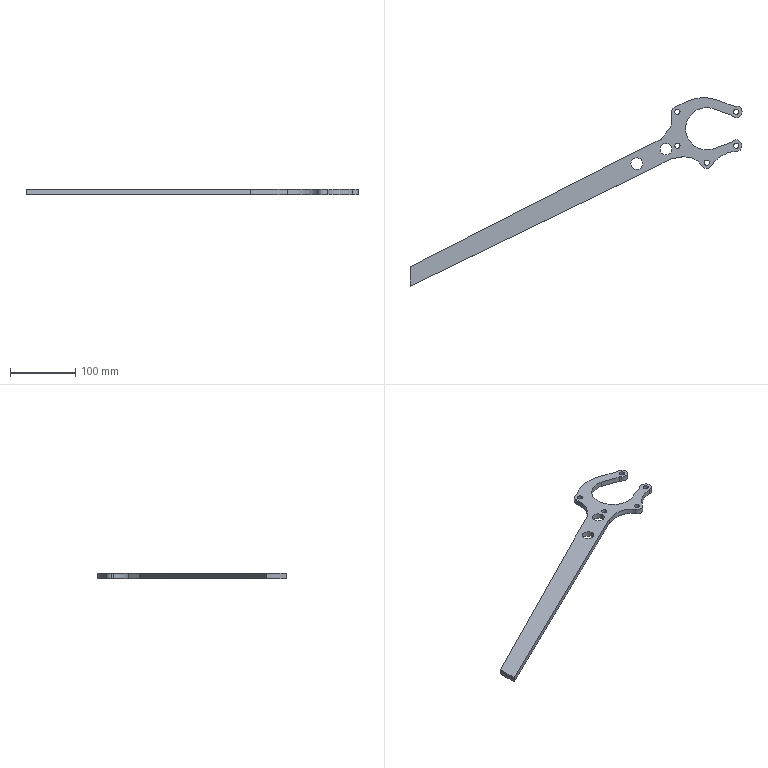Part | SolidWorks | features BaseBody 1 | 1 solid | 39 faces | box 509.458 x 289.148 x 8 mm | volume 145574 mm3 | cylinder 25 | plane 10 | spline 4 | commonest cylinder face diameters 8 x10 18 x9 20 x4 65 x2
STEP:
#1=CARTESIAN_POINT('',(-49.033,-26.,4.));
#2=VERTEX_POINT('',#1);
#3=CARTESIAN_POINT('',(-41.033,-26.,4.));
#4=VERTEX_POINT('',#3);
#5=CARTESIAN_POINT('',(-45.033,-26.,4.));
#6=DIRECTION('',(0.,0.,1.));
#7=DIRECTION('',(-1.,0.,0.));
#8=AXIS2_PLACEMENT_3D('',#5,#6,#7);
#9=CIRCLE('',#8,4.);
#10=EDGE_CURVE('',#2,#4,#9,.T.);
#11=ORIENTED_EDGE('',*,*,#10,.T.);
#12=CARTESIAN_POINT('',(-41.033,-26.,-4.));
#13=VERTEX_POINT('',#12);
#14=CARTESIAN_POINT('',(-41.033,-26.,4.));
#15=DIRECTION('',(0.,0.,-1.));
#16=VECTOR('',#15,1000.);
#17=LINE('',#14,#16);
#18=EDGE_CURVE('',#4,#13,#17,.T.);
#19=ORIENTED_EDGE('',*,*,#18,.T.);
#20=CARTESIAN_POINT('',(-49.033,-26.,-4.));
#21=VERTEX_POINT('',#20);
#22=CARTESIAN_POINT('',(-45.033,-26.,-4.));
#23=DIRECTION('',(0.,0.,-1.));
#24=DIRECTION('',(-1.,0.,0.));
#25=AXIS2_PLACEMENT_3D('',#22,#23,#24);
#26=CIRCLE('',#25,4.);
#27=EDGE_CURVE('',#13,#21,#26,.T.);
#28=ORIENTED_EDGE('',*,*,#27,.T.);
#29=CARTESIAN_POINT('',(-49.033,-26.,4.));
#30=DIRECTION('',(0.,0.,-1.));
#31=VECTOR('',#30,1000.);
#32=LINE('',#29,#31);
#33=EDGE_CURVE('',#2,#21,#32,.T.);
#34=ORIENTED_EDGE('',*,*,#33,.F.);
#35=EDGE_LOOP('',(#11,#19,#28,#34));
#36=FACE_OUTER_BOUND('',#35,.T.);
#37=CARTESIAN_POINT('',(-45.033,-26.,4.));
#38=DIRECTION('',(0.,0.,-1.));
#39=DIRECTION('',(-1.,0.,0.));
#40=AXIS2_PLACEMENT_3D('',#37,#38,#39);
#41=CYLINDRICAL_SURFACE('',#40,4.);
#42=ADVANCED_FACE('',(#36),#41,.F.);
#43=CARTESIAN_POINT('',(49.033,-26.,4.));
#44=VERTEX_POINT('',#43);
#45=CARTESIAN_POINT('',(41.033,-26.,4.));
#46=VERTEX_POINT('',#45);
#47=CARTESIAN_POINT('',(45.033,-26.,4.));
#48=DIRECTION('',(0.,0.,-1.));
#49=DIRECTION('',(-1.,0.,0.));
#50=AXIS2_PLACEMENT_3D('',#47,#48,#49);
#51=CIRCLE('',#50,4.);
#52=EDGE_CURVE('',#44,#46,#51,.T.);
#53=ORIENTED_EDGE('',*,*,#52,.F.);
#54=CARTESIAN_POINT('',(49.033,-26.,-4.));
#55=VERTEX_POINT('',#54);
#56=CARTESIAN_POINT('',(49.033,-26.,4.));
#57=DIRECTION('',(0.,0.,-1.));
#58=VECTOR('',#57,1000.);
#59=LINE('',#56,#58);
#60=EDGE_CURVE('',#44,#55,#59,.T.);
#61=ORIENTED_EDGE('',*,*,#60,.T.);
#62=CARTESIAN_POINT('',(41.033,-26.,-4.));
#63=VERTEX_POINT('',#62);
#64=CARTESIAN_POINT('',(45.033,-26.,-4.));
#65=DIRECTION('',(0.,0.,-1.));
#66=DIRECTION('',(-1.,0.,0.));
#67=AXIS2_PLACEMENT_3D('',#64,#65,#66);
#68=CIRCLE('',#67,4.);
#69=EDGE_CURVE('',#55,#63,#68,.T.);
#70=ORIENTED_EDGE('',*,*,#69,.T.);
#71=CARTESIAN_POINT('',(41.033,-26.,4.));
#72=DIRECTION('',(0.,0.,-1.));
#73=VECTOR('',#72,1000.);
#74=LINE('',#71,#73);
#75=EDGE_CURVE('',#46,#63,#74,.T.);
#76=ORIENTED_EDGE('',*,*,#75,.F.);
#77=EDGE_LOOP('',(#53,#61,#70,#76));
#78=FACE_OUTER_BOUND('',#77,.T.);
#79=CARTESIAN_POINT('',(45.033,-26.,4.));
#80=DIRECTION('',(0.,0.,-1.));
#81=DIRECTION('',(-1.,0.,0.));
#82=AXIS2_PLACEMENT_3D('',#79,#80,#81);
#83=CYLINDRICAL_SURFACE('',#82,4.);
#84=ADVANCED_FACE('',(#78),#83,.F.);
#85=CARTESIAN_POINT('',(4.,-52.,4.));
#86=VERTEX_POINT('',#85);
#87=CARTESIAN_POINT('',(-4.,-52.,4.));
#88=VERTEX_POINT('',#87);
#89=CARTESIAN_POINT('',(0.,-52.,4.));
#90=DIRECTION('',(0.,0.,-1.));
#91=DIRECTION('',(-1.,0.,0.));
#92=AXIS2_PLACEMENT_3D('',#89,#90,#91);
#93=CIRCLE('',#92,4.);
#94=EDGE_CURVE('',#86,#88,#93,.T.);
#95=ORIENTED_EDGE('',*,*,#94,.F.);
#96=CARTESIAN_POINT('',(4.,-52.,-4.));
#97=VERTEX_POINT('',#96);
#98=CARTESIAN_POINT('',(4.,-52.,4.));
#99=DIRECTION('',(0.,0.,-1.));
#100=VECTOR('',#99,1000.);
#101=LINE('',#98,#100);
#102=EDGE_CURVE('',#86,#97,#101,.T.);
#103=ORIENTED_EDGE('',*,*,#102,.T.);
#104=CARTESIAN_POINT('',(-4.,-52.,-4.));
#105=VERTEX_POINT('',#104);
#106=CARTESIAN_POINT('',(0.,-52.,-4.));
#107=DIRECTION('',(0.,0.,-1.));
#108=DIRECTION('',(-1.,0.,0.));
#109=AXIS2_PLACEMENT_3D('',#106,#107,#108);
#110=CIRCLE('',#109,4.);
#111=EDGE_CURVE('',#97,#105,#110,.T.);
#112=ORIENTED_EDGE('',*,*,#111,.T.);
#113=CARTESIAN_POINT('',(-4.,-52.,4.));
#114=DIRECTION('',(0.,0.,-1.));
#115=VECTOR('',#114,1000.);
#116=LINE('',#113,#115);
#117=EDGE_CURVE('',#88,#105,#116,.T.);
#118=ORIENTED_EDGE('',*,*,#117,.F.);
#119=EDGE_LOOP('',(#95,#103,#112,#118));
#120=FACE_OUTER_BOUND('',#119,.T.);
#121=CARTESIAN_POINT('',(0.,-52.,4.));
#122=DIRECTION('',(0.,0.,-1.));
#123=DIRECTION('',(-1.,0.,0.));
#124=AXIS2_PLACEMENT_3D('',#121,#122,#123);
#125=CYLINDRICAL_SURFACE('',#124,4.);
#126=ADVANCED_FACE('',(#120),#125,.F.);
#127=CARTESIAN_POINT('',(49.033,26.,4.));
#128=VERTEX_POINT('',#127);
#129=CARTESIAN_POINT('',(41.033,26.,4.));
#130=VERTEX_POINT('',#129);
#131=CARTESIAN_POINT('',(45.033,26.,4.));
#132=DIRECTION('',(0.,0.,-1.));
#133=DIRECTION('',(-1.,0.,0.));
#134=AXIS2_PLACEMENT_3D('',#131,#132,#133);
#135=CIRCLE('',#134,4.);
#136=EDGE_CURVE('',#128,#130,#135,.T.);
#137=ORIENTED_EDGE('',*,*,#136,.F.);
#138=CARTESIAN_POINT('',(49.033,26.,-4.));
#139=VERTEX_POINT('',#138);
#140=CARTESIAN_POINT('',(49.033,26.,4.));
#141=DIRECTION('',(0.,0.,-1.));
#142=VECTOR('',#141,1000.);
#143=LINE('',#140,#142);
#144=EDGE_CURVE('',#128,#139,#143,.T.);
#145=ORIENTED_EDGE('',*,*,#144,.T.);
#146=CARTESIAN_POINT('',(41.033,26.,-4.));
#147=VERTEX_POINT('',#146);
#148=CARTESIAN_POINT('',(45.033,26.,-4.));
#149=DIRECTION('',(0.,0.,-1.));
#150=DIRECTION('',(-1.,0.,0.));
#151=AXIS2_PLACEMENT_3D('',#148,#149,#150);
#152=CIRCLE('',#151,4.);
#153=EDGE_CURVE('',#139,#147,#152,.T.);
#154=ORIENTED_EDGE('',*,*,#153,.T.);
#155=CARTESIAN_POINT('',(41.033,26.,4.));
#156=DIRECTION('',(0.,0.,-1.));
#157=VECTOR('',#156,1000.);
#158=LINE('',#155,#157);
#159=EDGE_CURVE('',#130,#147,#158,.T.);
#160=ORIENTED_EDGE('',*,*,#159,.F.);
#161=EDGE_LOOP('',(#137,#145,#154,#160));
#162=FACE_OUTER_BOUND('',#161,.T.);
#163=CARTESIAN_POINT('',(45.033,26.,4.));
#164=DIRECTION('',(0.,0.,-1.));
#165=DIRECTION('',(-1.,0.,0.));
#166=AXIS2_PLACEMENT_3D('',#163,#164,#165);
#167=CYLINDRICAL_SURFACE('',#166,4.);
#168=ADVANCED_FACE('',(#162),#167,.F.);
#169=CARTESIAN_POINT('',(-41.033,26.,4.));
#170=VERTEX_POINT('',#169);
#171=CARTESIAN_POINT('',(-49.033,26.,4.));
#172=VERTEX_POINT('',#171);
#173=CARTESIAN_POINT('',(-45.033,26.,4.));
#174=DIRECTION('',(0.,0.,-1.));
#175=DIRECTION('',(-1.,0.,0.));
#176=AXIS2_PLACEMENT_3D('',#173,#174,#175);
#177=CIRCLE('',#176,4.);
#178=EDGE_CURVE('',#170,#172,#177,.T.);
#179=ORIENTED_EDGE('',*,*,#178,.F.);
#180=CARTESIAN_POINT('',(-41.033,26.,-4.));
#181=VERTEX_POINT('',#180);
#182=CARTESIAN_POINT('',(-41.033,26.,4.));
#183=DIRECTION('',(0.,0.,-1.));
#184=VECTOR('',#183,1000.);
#185=LINE('',#182,#184);
#186=EDGE_CURVE('',#170,#181,#185,.T.);
#187=ORIENTED_EDGE('',*,*,#186,.T.);
#188=CARTESIAN_POINT('',(-49.033,26.,-4.));
#189=VERTEX_POINT('',#188);
#190=CARTESIAN_POINT('',(-45.033,26.,-4.));
#191=DIRECTION('',(0.,0.,-1.));
#192=DIRECTION('',(-1.,0.,0.));
#193=AXIS2_PLACEMENT_3D('',#190,#191,#192);
#194=CIRCLE('',#193,4.);
#195=EDGE_CURVE('',#181,#189,#194,.T.);
#196=ORIENTED_EDGE('',*,*,#195,.T.);
#197=CARTESIAN_POINT('',(-49.033,26.,4.));
#198=DIRECTION('',(0.,0.,-1.));
#199=VECTOR('',#198,1000.);
#200=LINE('',#197,#199);
#201=EDGE_CURVE('',#172,#189,#200,.T.);
#202=ORIENTED_EDGE('',*,*,#201,.F.);
#203=EDGE_LOOP('',(#179,#187,#196,#202));
#204=FACE_OUTER_BOUND('',#203,.T.);
#205=CARTESIAN_POINT('',(-45.033,26.,4.));
#206=DIRECTION('',(0.,0.,-1.));
#207=DIRECTION('',(-1.,0.,0.));
#208=AXIS2_PLACEMENT_3D('',#205,#206,#207);
#209=CYLINDRICAL_SURFACE('',#208,4.);
#210=ADVANCED_FACE('',(#204),#209,.F.);
#211=CARTESIAN_POINT('',(-53.645,-31.234,4.));
#212=VERTEX_POINT('',#211);
#213=CARTESIAN_POINT('',(-71.645,-31.234,4.));
#214=VERTEX_POINT('',#213);
#215=CARTESIAN_POINT('',(-62.645,-31.234,4.));
#216=DIRECTION('',(0.,0.,-1.));
#217=DIRECTION('',(-1.,0.,0.));
#218=AXIS2_PLACEMENT_3D('',#215,#216,#217);
#219=CIRCLE('',#218,9.);
#220=EDGE_CURVE('',#212,#214,#219,.T.);
#221=ORIENTED_EDGE('',*,*,#220,.F.);
#222=CARTESIAN_POINT('',(-53.645,-31.234,-4.));
#223=VERTEX_POINT('',#222);
#224=CARTESIAN_POINT('',(-53.645,-31.234,4.));
#225=DIRECTION('',(0.,0.,-1.));
#226=VECTOR('',#225,1000.);
#227=LINE('',#224,#226);
#228=EDGE_CURVE('',#212,#223,#227,.T.);
#229=ORIENTED_EDGE('',*,*,#228,.T.);
#230=CARTESIAN_POINT('',(-71.645,-31.234,-4.));
#231=VERTEX_POINT('',#230);
#232=CARTESIAN_POINT('',(-62.645,-31.234,-4.));
#233=DIRECTION('',(0.,0.,-1.));
#234=DIRECTION('',(-1.,0.,0.));
#235=AXIS2_PLACEMENT_3D('',#232,#233,#234);
#236=CIRCLE('',#235,9.);
#237=EDGE_CURVE('',#223,#231,#236,.T.);
#238=ORIENTED_EDGE('',*,*,#237,.T.);
#239=CARTESIAN_POINT('',(-71.645,-31.234,4.));
#240=DIRECTION('',(0.,0.,-1.));
#241=VECTOR('',#240,1000.);
#242=LINE('',#239,#241);
#243=EDGE_CURVE('',#214,#231,#242,.T.);
#244=ORIENTED_EDGE('',*,*,#243,.F.);
#245=EDGE_LOOP('',(#221,#229,#238,#244));
#246=FACE_OUTER_BOUND('',#245,.T.);
#247=CARTESIAN_POINT('',(-62.645,-31.234,4.));
#248=DIRECTION('',(0.,0.,-1.));
#249=DIRECTION('',(-1.,0.,0.));
#250=AXIS2_PLACEMENT_3D('',#247,#248,#249);
#251=CYLINDRICAL_SURFACE('',#250,9.);
#252=ADVANCED_FACE('',(#246),#251,.F.);
#253=CARTESIAN_POINT('',(-98.392,-53.544,4.));
#254=VERTEX_POINT('',#253);
#255=CARTESIAN_POINT('',(-116.392,-53.544,4.));
#256=VERTEX_POINT('',#255);
#257=CARTESIAN_POINT('',(-107.392,-53.544,4.));
#258=DIRECTION('',(0.,0.,-1.));
#259=DIRECTION('',(-1.,0.,0.));
#260=AXIS2_PLACEMENT_3D('',#257,#258,#259);
#261=CIRCLE('',#260,9.);
#262=EDGE_CURVE('',#254,#256,#261,.T.);
#263=ORIENTED_EDGE('',*,*,#262,.F.);
#264=CARTESIAN_POINT('',(-98.392,-53.544,-4.));
#265=VERTEX_POINT('',#264);
#266=CARTESIAN_POINT('',(-98.392,-53.544,4.));
#267=DIRECTION('',(0.,0.,-1.));
#268=VECTOR('',#267,1000.);
#269=LINE('',#266,#268);
#270=EDGE_CURVE('',#254,#265,#269,.T.);
#271=ORIENTED_EDGE('',*,*,#270,.T.);
#272=CARTESIAN_POINT('',(-116.392,-53.544,-4.));
#273=VERTEX_POINT('',#272);
#274=CARTESIAN_POINT('',(-107.392,-53.544,-4.));
#275=DIRECTION('',(0.,0.,-1.));
#276=DIRECTION('',(-1.,0.,0.));
#277=AXIS2_PLACEMENT_3D('',#274,#275,#276);
#278=CIRCLE('',#277,9.);
#279=EDGE_CURVE('',#265,#273,#278,.T.);
#280=ORIENTED_EDGE('',*,*,#279,.T.);
#281=CARTESIAN_POINT('',(-116.392,-53.544,4.));
#282=DIRECTION('',(0.,0.,-1.));
#283=VECTOR('',#282,1000.);
#284=LINE('',#281,#283);
#285=EDGE_CURVE('',#256,#273,#284,.T.);
#286=ORIENTED_EDGE('',*,*,#285,.F.);
#287=EDGE_LOOP('',(#263,#271,#280,#286));
#288=FACE_OUTER_BOUND('',#287,.T.);
#289=CARTESIAN_POINT('',(-107.392,-53.544,4.));
#290=DIRECTION('',(0.,0.,-1.));
#291=DIRECTION('',(-1.,0.,0.));
#292=AXIS2_PLACEMENT_3D('',#289,#290,#291);
#293=CYLINDRICAL_SURFACE('',#292,9.);
#294=ADVANCED_FACE('',(#288),#293,.F.);
#295=CARTESIAN_POINT('',(-54.033,26.,4.));
#296=VERTEX_POINT('',#295);
#297=CARTESIAN_POINT('',(-53.834,24.118,4.));
#298=VERTEX_POINT('',#297);
#299=CARTESIAN_POINT('',(-45.033,26.,4.));
#300=DIRECTION('',(0.,0.,1.));
#301=DIRECTION('',(-1.,0.,0.));
#302=AXIS2_PLACEMENT_3D('',#299,#300,#301);
#303=CIRCLE('',#302,9.);
#304=EDGE_CURVE('',#296,#298,#303,.T.);
#305=ORIENTED_EDGE('',*,*,#304,.F.);
#306=CARTESIAN_POINT('',(-54.033,26.,-4.));
#307=VERTEX_POINT('',#306);
#308=CARTESIAN_POINT('',(-54.033,26.,4.));
#309=DIRECTION('',(0.,0.,-1.));
#310=VECTOR('',#309,1000.);
#311=LINE('',#308,#310);
#312=EDGE_CURVE('',#296,#307,#311,.T.);
#313=ORIENTED_EDGE('',*,*,#312,.T.);
#314=CARTESIAN_POINT('',(-53.834,24.118,-4.));
#315=VERTEX_POINT('',#314);
#316=CARTESIAN_POINT('',(-45.033,26.,-4.));
#317=DIRECTION('',(0.,0.,1.));
#318=DIRECTION('',(-1.,0.,0.));
#319=AXIS2_PLACEMENT_3D('',#316,#317,#318);
#320=CIRCLE('',#319,9.);
#321=EDGE_CURVE('',#307,#315,#320,.T.);
#322=ORIENTED_EDGE('',*,*,#321,.T.);
#323=CARTESIAN_POINT('',(-53.834,24.118,0.));
#324=DIRECTION('',(0.,0.,1.));
#325=VECTOR('',#324,1000.);
#326=LINE('',#323,#325);
#327=EDGE_CURVE('',#315,#298,#326,.T.);
#328=ORIENTED_EDGE('',*,*,#327,.T.);
#329=EDGE_LOOP('',(#305,#313,#322,#328));
#330=FACE_OUTER_BOUND('',#329,.T.);
#331=CARTESIAN_POINT('',(-45.033,26.,4.));
#332=DIRECTION('',(0.,0.,-1.));
#333=DIRECTION('',(-1.,0.,0.));
#334=AXIS2_PLACEMENT_3D('',#331,#332,#333);
#335=CYLINDRICAL_SURFACE('',#334,9.);
#336=ADVANCED_FACE('',(#330),#335,.T.);
#337=CARTESIAN_POINT('',(-32.5,0.,4.));
#338=VERTEX_POINT('',#337);
#339=CARTESIAN_POINT('',(6.433,31.857,4.));
#340=VERTEX_POINT('',#339);
#341=CARTESIAN_POINT('',(0.,0.,4.));
#342=DIRECTION('',(0.,0.,-1.));
#343=DIRECTION('',(-1.,0.,0.));
#344=AXIS2_PLACEMENT_3D('',#341,#342,#343);
#345=CIRCLE('',#344,32.5);
#346=EDGE_CURVE('',#338,#340,#345,.T.);
#347=ORIENTED_EDGE('',*,*,#346,.F.);
#348=CARTESIAN_POINT('',(-32.5,0.,-4.));
#349=VERTEX_POINT('',#348);
#350=CARTESIAN_POINT('',(-32.5,0.,4.));
#351=DIRECTION('',(0.,0.,-1.));
#352=VECTOR('',#351,1000.);
#353=LINE('',#350,#352);
#354=EDGE_CURVE('',#338,#349,#353,.T.);
#355=ORIENTED_EDGE('',*,*,#354,.T.);
#356=CARTESIAN_POINT('',(6.433,31.857,-4.));
#357=VERTEX_POINT('',#356);
#358=CARTESIAN_POINT('',(0.,0.,-4.));
#359=DIRECTION('',(0.,0.,-1.));
#360=DIRECTION('',(-1.,0.,0.));
#361=AXIS2_PLACEMENT_3D('',#358,#359,#360);
#362=CIRCLE('',#361,32.5);
#363=EDGE_CURVE('',#349,#357,#362,.T.);
#364=ORIENTED_EDGE('',*,*,#363,.T.);
#365=CARTESIAN_POINT('',(6.433,31.857,0.));
#366=DIRECTION('',(0.,0.,-1.));
#367=VECTOR('',#366,1000.);
#368=LINE('',#365,#367);
#369=EDGE_CURVE('',#340,#357,#368,.T.);
#370=ORIENTED_EDGE('',*,*,#369,.F.);
#371=EDGE_LOOP('',(#347,#355,#364,#370));
#372=FACE_OUTER_BOUND('',#371,.T.);
#373=CARTESIAN_POINT('',(0.,0.,4.));
#374=DIRECTION('',(0.,0.,-1.));
#375=DIRECTION('',(-1.,0.,0.));
#376=AXIS2_PLACEMENT_3D('',#373,#374,#375);
#377=CYLINDRICAL_SURFACE('',#376,32.5);
#378=ADVANCED_FACE('',(#372),#377,.F.);
#379=ORIENTED_EDGE('',*,*,#18,.F.);
#380=CARTESIAN_POINT('',(-45.033,-26.,4.));
#381=DIRECTION('',(0.,0.,1.));
#382=DIRECTION('',(-1.,0.,0.));
#383=AXIS2_PLACEMENT_3D('',#380,#381,#382);
#384=CIRCLE('',#383,4.);
#385=EDGE_CURVE('',#4,#2,#384,.T.);
#386=ORIENTED_EDGE('',*,*,#385,.T.);
#387=ORIENTED_EDGE('',*,*,#33,.T.);
#388=CARTESIAN_POINT('',(-45.033,-26.,-4.));
#389=DIRECTION('',(0.,0.,-1.));
#390=DIRECTION('',(-1.,0.,0.));
#391=AXIS2_PLACEMENT_3D('',#388,#389,#390);
#392=CIRCLE('',#391,4.);
#393=EDGE_CURVE('',#21,#13,#392,.T.);
#394=ORIENTED_EDGE('',*,*,#393,.T.);
#395=EDGE_LOOP('',(#379,#386,#387,#394));
#396=FACE_OUTER_BOUND('',#395,.T.);
#397=CARTESIAN_POINT('',(-45.033,-26.,4.));
#398=DIRECTION('',(0.,0.,-1.));
#399=DIRECTION('',(-1.,0.,0.));
#400=AXIS2_PLACEMENT_3D('',#397,#398,#399);
#401=CYLINDRICAL_SURFACE('',#400,4.);
#402=ADVANCED_FACE('',(#396),#401,.F.);
#403=ORIENTED_EDGE('',*,*,#393,.F.);
#404=ORIENTED_EDGE('',*,*,#27,.F.);
#405=EDGE_LOOP('',(#403,#404));
#406=FACE_BOUND('',#405,.T.);
#407=CARTESIAN_POINT('',(45.033,-26.,-4.));
#408=DIRECTION('',(0.,0.,-1.));
#409=DIRECTION('',(-1.,0.,0.));
#410=AXIS2_PLACEMENT_3D('',#407,#408,#409);
#411=CIRCLE('',#410,4.);
#412=EDGE_CURVE('',#63,#55,#411,.T.);
#413=ORIENTED_EDGE('',*,*,#412,.F.);
#414=ORIENTED_EDGE('',*,*,#69,.F.);
#415=EDGE_LOOP('',(#413,#414));
#416=FACE_BOUND('',#415,.T.);
#417=CARTESIAN_POINT('',(0.,-52.,-4.));
#418=DIRECTION('',(0.,0.,-1.));
#419=DIRECTION('',(-1.,0.,0.));
#420=AXIS2_PLACEMENT_3D('',#417,#418,#419);
#421=CIRCLE('',#420,4.);
#422=EDGE_CURVE('',#105,#97,#421,.T.);
#423=ORIENTED_EDGE('',*,*,#422,.F.);
#424=ORIENTED_EDGE('',*,*,#111,.F.);
#425=EDGE_LOOP('',(#423,#424));
#426=FACE_BOUND('',#425,.T.);
#427=CARTESIAN_POINT('',(45.033,26.,-4.));
#428=DIRECTION('',(0.,0.,-1.));
#429=DIRECTION('',(-1.,0.,0.));
#430=AXIS2_PLACEMENT_3D('',#427,#428,#429);
#431=CIRCLE('',#430,4.);
#432=EDGE_CURVE('',#147,#139,#431,.T.);
#433=ORIENTED_EDGE('',*,*,#432,.F.);
#434=ORIENTED_EDGE('',*,*,#153,.F.);
#435=EDGE_LOOP('',(#433,#434));
#436=FACE_BOUND('',#435,.T.);
#437=CARTESIAN_POINT('',(-45.033,26.,-4.));
#438=DIRECTION('',(0.,0.,-1.));
#439=DIRECTION('',(-1.,0.,0.));
#440=AXIS2_PLACEMENT_3D('',#437,#438,#439);
#441=CIRCLE('',#440,4.);
#442=EDGE_CURVE('',#189,#181,#441,.T.);
#443=ORIENTED_EDGE('',*,*,#442,.F.);
#444=ORIENTED_EDGE('',*,*,#195,.F.);
#445=EDGE_LOOP('',(#443,#444));
#446=FACE_BOUND('',#445,.T.);
#447=CARTESIAN_POINT('',(-62.645,-31.234,-4.));
#448=DIRECTION('',(0.,0.,-1.));
#449=DIRECTION('',(-1.,0.,0.));
#450=AXIS2_PLACEMENT_3D('',#447,#448,#449);
#451=CIRCLE('',#450,9.);
#452=EDGE_CURVE('',#231,#223,#451,.T.);
#453=ORIENTED_EDGE('',*,*,#452,.F.);
#454=ORIENTED_EDGE('',*,*,#237,.F.);
#455=EDGE_LOOP('',(#453,#454));
#456=FACE_BOUND('',#455,.T.);
#457=CARTESIAN_POINT('',(-107.392,-53.544,-4.));
#458=DIRECTION('',(0.,0.,-1.));
#459=DIRECTION('',(-1.,0.,0.));
#460=AXIS2_PLACEMENT_3D('',#457,#458,#459);
#461=CIRCLE('',#460,9.);
#462=EDGE_CURVE('',#273,#265,#461,.T.);
#463=ORIENTED_EDGE('',*,*,#462,.F.);
#464=ORIENTED_EDGE('',*,*,#279,.F.);
#465=EDGE_LOOP('',(#463,#464));
#466=FACE_BOUND('',#465,.T.);
#467=CARTESIAN_POINT('',(-455.373,-211.538,-4.));
#468=VERTEX_POINT('',#467);
#469=CARTESIAN_POINT('',(-455.425,-241.465,-4.));
#470=VERTEX_POINT('',#469);
#471=CARTESIAN_POINT('',(-455.425,-241.465,-4.));
#472=DIRECTION('',(-0.001745,-1.,0.));
#473=VECTOR('',#472,1000.);
#474=LINE('',#471,#473);
#475=EDGE_CURVE('',#468,#470,#474,.T.);
#476=ORIENTED_EDGE('',*,*,#475,.F.);
#477=CARTESIAN_POINT('',(-127.298,-44.473,-4.));
#478=VERTEX_POINT('',#477);
#479=CARTESIAN_POINT('',(-455.373,-211.538,-4.));
#480=DIRECTION('',(-0.8911,-0.4538,0.));
#481=VECTOR('',#480,1000.);
#482=LINE('',#479,#481);
#483=EDGE_CURVE('',#478,#468,#482,.T.);
#484=ORIENTED_EDGE('',*,*,#483,.F.);
#485=CARTESIAN_POINT('',(-70.231,-16.02,-4.));
#486=VERTEX_POINT('',#485);
#487=CARTESIAN_POINT('',(-127.298,-44.473,-4.));
#488=DIRECTION('',(-0.8949,-0.4462,0.));
#489=VECTOR('',#488,1000.);
#490=LINE('',#487,#489);
#491=EDGE_CURVE('',#486,#478,#490,.T.);
#492=ORIENTED_EDGE('',*,*,#491,.F.);
#493=CARTESIAN_POINT('',(-57.174,-0.000000019,-4.));
#494=VERTEX_POINT('',#493);
#495=CARTESIAN_POINT('',(-57.174,0.,-4.));
#496=DIRECTION('',(-0.6318,-0.7751,0.));
#497=VECTOR('',#496,1000.);
#498=LINE('',#495,#497);
#499=EDGE_CURVE('',#494,#486,#498,.T.);
#500=ORIENTED_EDGE('',*,*,#499,.F.);
#501=CARTESIAN_POINT('',(-53.834,24.118,-4.));
#502=CARTESIAN_POINT('',(-52.682,12.031,-4.));
#503=CARTESIAN_POINT('',(-54.081,5.475,-4.));
#504=CARTESIAN_POINT('',(-57.174,-0.000000019,-4.));
#505=B_SPLINE_CURVE_WITH_KNOTS('',3,(#501,#502,#503,#504),.UNSPECIFIED.,.F.,.F.,(4,4),(0.,0.02481),.UNSPECIFIED.);
#506=EDGE_CURVE('',#315,#494,#505,.T.);
#507=ORIENTED_EDGE('',*,*,#506,.F.);
#508=ORIENTED_EDGE('',*,*,#321,.F.);
#509=CARTESIAN_POINT('',(-46.406,34.895,-4.));
#510=VERTEX_POINT('',#509);
#511=CARTESIAN_POINT('',(-45.033,26.,-4.));
#512=DIRECTION('',(0.,0.,1.));
#513=DIRECTION('',(-1.,0.,0.));
#514=AXIS2_PLACEMENT_3D('',#511,#512,#513);
#515=CIRCLE('',#514,9.);
#516=EDGE_CURVE('',#510,#307,#515,.T.);
#517=ORIENTED_EDGE('',*,*,#516,.F.);
#518=CARTESIAN_POINT('',(-43.301,35.914,-4.));
#519=VERTEX_POINT('',#518);
#520=CARTESIAN_POINT('',(-47.93,44.778,-4.));
#521=DIRECTION('',(0.,0.,-1.));
#522=DIRECTION('',(-1.,0.,0.));
#523=AXIS2_PLACEMENT_3D('',#520,#521,#522);
#524=CIRCLE('',#523,10.);
#525=EDGE_CURVE('',#519,#510,#524,.T.);
#526=ORIENTED_EDGE('',*,*,#525,.F.);
#527=CARTESIAN_POINT('',(38.851,35.688,-4.));
#528=VERTEX_POINT('',#527);
#529=CARTESIAN_POINT('',(38.851,35.688,-4.));
#530=CARTESIAN_POINT('',(20.692,43.525,-4.));
#531=CARTESIAN_POINT('',(-4.612,51.647,-4.));
#532=CARTESIAN_POINT('',(-28.001,43.905,-4.));
#533=CARTESIAN_POINT('',(-43.301,35.914,-4.));
#534=B_SPLINE_CURVE_WITH_KNOTS('',3,(#529,#530,#531,#532,#533),.UNSPECIFIED.,.F.,.F.,(4,1,4),(0.,0.04398,0.08638),.UNSPECIFIED.);
#535=EDGE_CURVE('',#528,#519,#534,.T.);
#536=ORIENTED_EDGE('',*,*,#535,.F.);
#537=CARTESIAN_POINT('',(43.982,34.938,-4.));
#538=VERTEX_POINT('',#537);
#539=CARTESIAN_POINT('',(42.813,44.87,-4.));
#540=DIRECTION('',(0.,0.,-1.));
#541=DIRECTION('',(-1.,0.,0.));
#542=AXIS2_PLACEMENT_3D('',#539,#540,#541);
#543=CIRCLE('',#542,10.);
#544=EDGE_CURVE('',#538,#528,#543,.T.);
#545=ORIENTED_EDGE('',*,*,#544,.F.);
#546=CARTESIAN_POINT('',(38.803,19.506,-4.));
#547=VERTEX_POINT('',#546);
#548=CARTESIAN_POINT('',(45.033,26.,-4.));
#549=DIRECTION('',(0.,0.,1.));
#550=DIRECTION('',(-1.,0.,0.));
#551=AXIS2_PLACEMENT_3D('',#548,#549,#550);
#552=CIRCLE('',#551,9.);
#553=EDGE_CURVE('',#547,#538,#552,.T.);
#554=ORIENTED_EDGE('',*,*,#553,.F.);
#555=CARTESIAN_POINT('',(35.202,21.721,-4.));
#556=VERTEX_POINT('',#555);
#557=CARTESIAN_POINT('',(31.879,12.29,-4.));
#558=DIRECTION('',(0.,0.,-1.));
#559=DIRECTION('',(-1.,0.,0.));
#560=AXIS2_PLACEMENT_3D('',#557,#558,#559);
#561=CIRCLE('',#560,10.);
#562=EDGE_CURVE('',#556,#547,#561,.T.);
#563=ORIENTED_EDGE('',*,*,#562,.F.);
#564=CARTESIAN_POINT('',(6.433,31.857,-4.));
#565=DIRECTION('',(0.9432,-0.3323,0.));
#566=VECTOR('',#565,1000.);
#567=LINE('',#564,#566);
#568=EDGE_CURVE('',#357,#556,#567,.T.);
#569=ORIENTED_EDGE('',*,*,#568,.F.);
#570=ORIENTED_EDGE('',*,*,#363,.F.);
#571=CARTESIAN_POINT('',(6.433,-31.857,-4.));
#572=VERTEX_POINT('',#571);
#573=CARTESIAN_POINT('',(0.,0.,-4.));
#574=DIRECTION('',(0.,0.,-1.));
#575=DIRECTION('',(-1.,0.,0.));
#576=AXIS2_PLACEMENT_3D('',#573,#574,#575);
#577=CIRCLE('',#576,32.5);
#578=EDGE_CURVE('',#572,#349,#577,.T.);
#579=ORIENTED_EDGE('',*,*,#578,.F.);
#580=CARTESIAN_POINT('',(35.202,-21.721,-4.));
#581=VERTEX_POINT('',#580);
#582=CARTESIAN_POINT('',(6.433,-31.857,-4.));
#583=DIRECTION('',(-0.9432,-0.3323,0.));
#584=VECTOR('',#583,1000.);
#585=LINE('',#582,#584);
#586=EDGE_CURVE('',#581,#572,#585,.T.);
#587=ORIENTED_EDGE('',*,*,#586,.F.);
#588=CARTESIAN_POINT('',(38.803,-19.506,-4.));
#589=VERTEX_POINT('',#588);
#590=CARTESIAN_POINT('',(31.879,-12.29,-4.));
#591=DIRECTION('',(0.,0.,-1.));
#592=DIRECTION('',(-1.,0.,0.));
#593=AXIS2_PLACEMENT_3D('',#590,#591,#592);
#594=CIRCLE('',#593,10.);
#595=EDGE_CURVE('',#589,#581,#594,.T.);
#596=ORIENTED_EDGE('',*,*,#595,.F.);
#597=CARTESIAN_POINT('',(45.033,-35.,-4.));
#598=VERTEX_POINT('',#597);
#599=CARTESIAN_POINT('',(45.033,-26.,-4.));
#600=DIRECTION('',(0.,0.,1.));
#601=DIRECTION('',(-1.,0.,0.));
#602=AXIS2_PLACEMENT_3D('',#599,#600,#601);
#603=CIRCLE('',#602,9.);
#604=EDGE_CURVE('',#598,#589,#603,.T.);
#605=ORIENTED_EDGE('',*,*,#604,.F.);
#606=CARTESIAN_POINT('',(7.645,-56.75,-4.));
#607=VERTEX_POINT('',#606);
#608=CARTESIAN_POINT('',(7.645,-56.75,-4.));
#609=CARTESIAN_POINT('',(14.185,-43.649,-4.));
#610=CARTESIAN_POINT('',(30.699,-34.916,-4.));
#611=CARTESIAN_POINT('',(45.033,-35.,-4.));
#612=B_SPLINE_CURVE_WITH_KNOTS('',3,(#608,#609,#610,#611),.UNSPECIFIED.,.F.,.F.,(4,4),(0.,0.04517),.UNSPECIFIED.);
#613=EDGE_CURVE('',#607,#598,#612,.T.);
#614=ORIENTED_EDGE('',*,*,#613,.F.);
#615=CARTESIAN_POINT('',(-7.645,-56.75,-4.));
#616=VERTEX_POINT('',#615);
#617=CARTESIAN_POINT('',(0.,-52.,-4.));
#618=DIRECTION('',(0.,0.,1.));
#619=DIRECTION('',(-1.,0.,0.));
#620=AXIS2_PLACEMENT_3D('',#617,#618,#619);
#621=CIRCLE('',#620,9.);
#622=EDGE_CURVE('',#616,#607,#621,.T.);
#623=ORIENTED_EDGE('',*,*,#622,.F.);
#624=CARTESIAN_POINT('',(-54.648,-46.242,-4.));
#625=VERTEX_POINT('',#624);
#626=CARTESIAN_POINT('',(-54.648,-46.242,-4.));
#627=CARTESIAN_POINT('',(-20.324,-36.229,-4.));
#628=CARTESIAN_POINT('',(-7.645,-56.75,-4.));
#629=B_SPLINE_CURVE_WITH_KNOTS('',2,(#626,#627,#628),.UNSPECIFIED.,.F.,.F.,(3,3),(0.,0.05204),.UNSPECIFIED.);
#630=EDGE_CURVE('',#625,#616,#629,.T.);
#631=ORIENTED_EDGE('',*,*,#630,.F.);
#632=CARTESIAN_POINT('',(-111.085,-74.381,-4.));
#633=VERTEX_POINT('',#632);
#634=CARTESIAN_POINT('',(-111.085,-74.381,-4.));
#635=DIRECTION('',(0.8949,0.4462,0.));
#636=VECTOR('',#635,1000.);
#637=LINE('',#634,#636);
#638=EDGE_CURVE('',#633,#625,#637,.T.);
#639=ORIENTED_EDGE('',*,*,#638,.F.);
#640=CARTESIAN_POINT('',(-455.425,-241.465,-4.));
#641=DIRECTION('',(0.8997,0.4366,0.));
#642=VECTOR('',#641,1000.);
#643=LINE('',#640,#642);
#644=EDGE_CURVE('',#470,#633,#643,.T.);
#645=ORIENTED_EDGE('',*,*,#644,.F.);
#646=EDGE_LOOP('',(#476,#484,#492,#500,#507,#508,#517,#526,#536,#545,#554,#563,#569,#570,#579,#587,#596,#605,#614,#623,#631,#639,#645));
#647=FACE_OUTER_BOUND('',#646,.T.);
#648=CARTESIAN_POINT('',(-458.482,-243.201,-4.));
#649=DIRECTION('',(0.,0.,1.));
#650=DIRECTION('',(1.,0.,0.));
#651=AXIS2_PLACEMENT_3D('',#648,#649,#650);
#652=PLANE('',#651);
#653=ADVANCED_FACE('',(#406,#416,#426,#436,#446,#456,#466,#647),#652,.F.);
#654=ORIENTED_EDGE('',*,*,#10,.F.);
#655=ORIENTED_EDGE('',*,*,#385,.F.);
#656=EDGE_LOOP('',(#654,#655));
#657=FACE_BOUND('',#656,.T.);
#658=CARTESIAN_POINT('',(45.033,-26.,4.));
#659=DIRECTION('',(0.,0.,-1.));
#660=DIRECTION('',(-1.,0.,0.));
#661=AXIS2_PLACEMENT_3D('',#658,#659,#660);
#662=CIRCLE('',#661,4.);
#663=EDGE_CURVE('',#46,#44,#662,.T.);
#664=ORIENTED_EDGE('',*,*,#663,.T.);
#665=ORIENTED_EDGE('',*,*,#52,.T.);
#666=EDGE_LOOP('',(#664,#665));
#667=FACE_BOUND('',#666,.T.);
#668=CARTESIAN_POINT('',(0.,-52.,4.));
#669=DIRECTION('',(0.,0.,-1.));
#670=DIRECTION('',(-1.,0.,0.));
#671=AXIS2_PLACEMENT_3D('',#668,#669,#670);
#672=CIRCLE('',#671,4.);
#673=EDGE_CURVE('',#88,#86,#672,.T.);
#674=ORIENTED_EDGE('',*,*,#673,.T.);
#675=ORIENTED_EDGE('',*,*,#94,.T.);
#676=EDGE_LOOP('',(#674,#675));
#677=FACE_BOUND('',#676,.T.);
#678=CARTESIAN_POINT('',(45.033,26.,4.));
#679=DIRECTION('',(0.,0.,-1.));
#680=DIRECTION('',(-1.,0.,0.));
#681=AXIS2_PLACEMENT_3D('',#678,#679,#680);
#682=CIRCLE('',#681,4.);
#683=EDGE_CURVE('',#130,#128,#682,.T.);
#684=ORIENTED_EDGE('',*,*,#683,.T.);
#685=ORIENTED_EDGE('',*,*,#136,.T.);
#686=EDGE_LOOP('',(#684,#685));
#687=FACE_BOUND('',#686,.T.);
#688=CARTESIAN_POINT('',(-45.033,26.,4.));
#689=DIRECTION('',(0.,0.,-1.));
#690=DIRECTION('',(-1.,0.,0.));
#691=AXIS2_PLACEMENT_3D('',#688,#689,#690);
#692=CIRCLE('',#691,4.);
#693=EDGE_CURVE('',#172,#170,#692,.T.);
#694=ORIENTED_EDGE('',*,*,#693,.T.);
#695=ORIENTED_EDGE('',*,*,#178,.T.);
#696=EDGE_LOOP('',(#694,#695));
#697=FACE_BOUND('',#696,.T.);
#698=CARTESIAN_POINT('',(-62.645,-31.234,4.));
#699=DIRECTION('',(0.,0.,-1.));
#700=DIRECTION('',(-1.,0.,0.));
#701=AXIS2_PLACEMENT_3D('',#698,#699,#700);
#702=CIRCLE('',#701,9.);
#703=EDGE_CURVE('',#214,#212,#702,.T.);
#704=ORIENTED_EDGE('',*,*,#703,.T.);
#705=ORIENTED_EDGE('',*,*,#220,.T.);
#706=EDGE_LOOP('',(#704,#705));
#707=FACE_BOUND('',#706,.T.);
#708=CARTESIAN_POINT('',(-107.392,-53.544,4.));
#709=DIRECTION('',(0.,0.,-1.));
#710=DIRECTION('',(-1.,0.,0.));
#711=AXIS2_PLACEMENT_3D('',#708,#709,#710);
#712=CIRCLE('',#711,9.);
#713=EDGE_CURVE('',#256,#254,#712,.T.);
#714=ORIENTED_EDGE('',*,*,#713,.T.);
#715=ORIENTED_EDGE('',*,*,#262,.T.);
#716=EDGE_LOOP('',(#714,#715));
#717=FACE_BOUND('',#716,.T.);
#718=CARTESIAN_POINT('',(-70.231,-16.02,4.));
#719=VERTEX_POINT('',#718);
#720=CARTESIAN_POINT('',(-127.298,-44.473,4.));
#721=VERTEX_POINT('',#720);
#722=CARTESIAN_POINT('',(-70.231,-16.02,4.));
#723=DIRECTION('',(-0.8949,-0.4462,0.));
#724=VECTOR('',#723,1000.);
#725=LINE('',#722,#724);
#726=EDGE_CURVE('',#719,#721,#725,.T.);
#727=ORIENTED_EDGE('',*,*,#726,.T.);
#728=CARTESIAN_POINT('',(-455.373,-211.538,4.));
#729=VERTEX_POINT('',#728);
#730=CARTESIAN_POINT('',(-127.298,-44.473,4.));
#731=DIRECTION('',(-0.8911,-0.4538,0.));
#732=VECTOR('',#731,1000.);
#733=LINE('',#730,#732);
#734=EDGE_CURVE('',#721,#729,#733,.T.);
#735=ORIENTED_EDGE('',*,*,#734,.T.);
#736=CARTESIAN_POINT('',(-455.425,-241.465,4.));
#737=VERTEX_POINT('',#736);
#738=CARTESIAN_POINT('',(-455.373,-211.538,4.));
#739=DIRECTION('',(-0.001745,-1.,0.));
#740=VECTOR('',#739,1000.);
#741=LINE('',#738,#740);
#742=EDGE_CURVE('',#729,#737,#741,.T.);
#743=ORIENTED_EDGE('',*,*,#742,.T.);
#744=CARTESIAN_POINT('',(-111.085,-74.381,4.));
#745=VERTEX_POINT('',#744);
#746=CARTESIAN_POINT('',(-455.425,-241.465,4.));
#747=DIRECTION('',(0.8997,0.4366,0.));
#748=VECTOR('',#747,1000.);
#749=LINE('',#746,#748);
#750=EDGE_CURVE('',#737,#745,#749,.T.);
#751=ORIENTED_EDGE('',*,*,#750,.T.);
#752=CARTESIAN_POINT('',(-54.648,-46.242,4.));
#753=VERTEX_POINT('',#752);
#754=CARTESIAN_POINT('',(-111.085,-74.381,4.));
#755=DIRECTION('',(0.8949,0.4462,0.));
#756=VECTOR('',#755,1000.);
#757=LINE('',#754,#756);
#758=EDGE_CURVE('',#745,#753,#757,.T.);
#759=ORIENTED_EDGE('',*,*,#758,.T.);
#760=CARTESIAN_POINT('',(-7.645,-56.75,4.));
#761=VERTEX_POINT('',#760);
#762=CARTESIAN_POINT('',(-54.648,-46.242,4.));
#763=CARTESIAN_POINT('',(-20.324,-36.229,4.));
#764=CARTESIAN_POINT('',(-7.645,-56.75,4.));
#765=B_SPLINE_CURVE_WITH_KNOTS('',2,(#762,#763,#764),.UNSPECIFIED.,.F.,.F.,(3,3),(0.,0.05204),.UNSPECIFIED.);
#766=EDGE_CURVE('',#753,#761,#765,.T.);
#767=ORIENTED_EDGE('',*,*,#766,.T.);
#768=CARTESIAN_POINT('',(7.645,-56.75,4.));
#769=VERTEX_POINT('',#768);
#770=CARTESIAN_POINT('',(0.,-52.,4.));
#771=DIRECTION('',(0.,0.,1.));
#772=DIRECTION('',(-1.,0.,0.));
#773=AXIS2_PLACEMENT_3D('',#770,#771,#772);
#774=CIRCLE('',#773,9.);
#775=EDGE_CURVE('',#761,#769,#774,.T.);
#776=ORIENTED_EDGE('',*,*,#775,.T.);
#777=CARTESIAN_POINT('',(45.033,-35.,4.));
#778=VERTEX_POINT('',#777);
#779=CARTESIAN_POINT('',(7.645,-56.75,4.));
#780=CARTESIAN_POINT('',(14.185,-43.649,4.));
#781=CARTESIAN_POINT('',(30.699,-34.916,4.));
#782=CARTESIAN_POINT('',(45.033,-35.,4.));
#783=B_SPLINE_CURVE_WITH_KNOTS('',3,(#779,#780,#781,#782),.UNSPECIFIED.,.F.,.F.,(4,4),(0.,0.04517),.UNSPECIFIED.);
#784=EDGE_CURVE('',#769,#778,#783,.T.);
#785=ORIENTED_EDGE('',*,*,#784,.T.);
#786=CARTESIAN_POINT('',(38.803,-19.506,4.));
#787=VERTEX_POINT('',#786);
#788=CARTESIAN_POINT('',(45.033,-26.,4.));
#789=DIRECTION('',(0.,0.,1.));
#790=DIRECTION('',(-1.,0.,0.));
#791=AXIS2_PLACEMENT_3D('',#788,#789,#790);
#792=CIRCLE('',#791,9.);
#793=EDGE_CURVE('',#778,#787,#792,.T.);
#794=ORIENTED_EDGE('',*,*,#793,.T.);
#795=CARTESIAN_POINT('',(35.202,-21.721,4.));
#796=VERTEX_POINT('',#795);
#797=CARTESIAN_POINT('',(31.879,-12.29,4.));
#798=DIRECTION('',(0.,0.,-1.));
#799=DIRECTION('',(-1.,0.,0.));
#800=AXIS2_PLACEMENT_3D('',#797,#798,#799);
#801=CIRCLE('',#800,10.);
#802=EDGE_CURVE('',#787,#796,#801,.T.);
#803=ORIENTED_EDGE('',*,*,#802,.T.);
#804=CARTESIAN_POINT('',(6.433,-31.857,4.));
#805=VERTEX_POINT('',#804);
#806=CARTESIAN_POINT('',(35.202,-21.721,4.));
#807=DIRECTION('',(-0.9432,-0.3323,0.));
#808=VECTOR('',#807,1000.);
#809=LINE('',#806,#808);
#810=EDGE_CURVE('',#796,#805,#809,.T.);
#811=ORIENTED_EDGE('',*,*,#810,.T.);
#812=CARTESIAN_POINT('',(0.,0.,4.));
#813=DIRECTION('',(0.,0.,-1.));
#814=DIRECTION('',(-1.,0.,0.));
#815=AXIS2_PLACEMENT_3D('',#812,#813,#814);
#816=CIRCLE('',#815,32.5);
#817=EDGE_CURVE('',#805,#338,#816,.T.);
#818=ORIENTED_EDGE('',*,*,#817,.T.);
#819=ORIENTED_EDGE('',*,*,#346,.T.);
#820=CARTESIAN_POINT('',(35.202,21.721,4.));
#821=VERTEX_POINT('',#820);
#822=CARTESIAN_POINT('',(6.433,31.857,4.));
#823=DIRECTION('',(0.9432,-0.3323,0.));
#824=VECTOR('',#823,1000.);
#825=LINE('',#822,#824);
#826=EDGE_CURVE('',#340,#821,#825,.T.);
#827=ORIENTED_EDGE('',*,*,#826,.T.);
#828=CARTESIAN_POINT('',(38.803,19.506,4.));
#829=VERTEX_POINT('',#828);
#830=CARTESIAN_POINT('',(31.879,12.29,4.));
#831=DIRECTION('',(0.,0.,-1.));
#832=DIRECTION('',(-1.,0.,0.));
#833=AXIS2_PLACEMENT_3D('',#830,#831,#832);
#834=CIRCLE('',#833,10.);
#835=EDGE_CURVE('',#821,#829,#834,.T.);
#836=ORIENTED_EDGE('',*,*,#835,.T.);
#837=CARTESIAN_POINT('',(43.982,34.938,4.));
#838=VERTEX_POINT('',#837);
#839=CARTESIAN_POINT('',(45.033,26.,4.));
#840=DIRECTION('',(0.,0.,1.));
#841=DIRECTION('',(-1.,0.,0.));
#842=AXIS2_PLACEMENT_3D('',#839,#840,#841);
#843=CIRCLE('',#842,9.);
#844=EDGE_CURVE('',#829,#838,#843,.T.);
#845=ORIENTED_EDGE('',*,*,#844,.T.);
#846=CARTESIAN_POINT('',(38.851,35.688,4.));
#847=VERTEX_POINT('',#846);
#848=CARTESIAN_POINT('',(42.813,44.87,4.));
#849=DIRECTION('',(0.,0.,-1.));
#850=DIRECTION('',(-1.,0.,0.));
#851=AXIS2_PLACEMENT_3D('',#848,#849,#850);
#852=CIRCLE('',#851,10.);
#853=EDGE_CURVE('',#838,#847,#852,.T.);
#854=ORIENTED_EDGE('',*,*,#853,.T.);
#855=CARTESIAN_POINT('',(-43.301,35.914,4.));
#856=VERTEX_POINT('',#855);
#857=CARTESIAN_POINT('',(38.851,35.688,4.));
#858=CARTESIAN_POINT('',(20.692,43.525,4.));
#859=CARTESIAN_POINT('',(-4.612,51.647,4.));
#860=CARTESIAN_POINT('',(-28.001,43.905,4.));
#861=CARTESIAN_POINT('',(-43.301,35.914,4.));
#862=B_SPLINE_CURVE_WITH_KNOTS('',3,(#857,#858,#859,#860,#861),.UNSPECIFIED.,.F.,.F.,(4,1,4),(0.,0.04398,0.08638),.UNSPECIFIED.);
#863=EDGE_CURVE('',#847,#856,#862,.T.);
#864=ORIENTED_EDGE('',*,*,#863,.T.);
#865=CARTESIAN_POINT('',(-46.406,34.895,4.));
#866=VERTEX_POINT('',#865);
#867=CARTESIAN_POINT('',(-47.93,44.778,4.));
#868=DIRECTION('',(0.,0.,-1.));
#869=DIRECTION('',(-1.,0.,0.));
#870=AXIS2_PLACEMENT_3D('',#867,#868,#869);
#871=CIRCLE('',#870,10.);
#872=EDGE_CURVE('',#856,#866,#871,.T.);
#873=ORIENTED_EDGE('',*,*,#872,.T.);
#874=CARTESIAN_POINT('',(-45.033,26.,4.));
#875=DIRECTION('',(0.,0.,1.));
#876=DIRECTION('',(-1.,0.,0.));
#877=AXIS2_PLACEMENT_3D('',#874,#875,#876);
#878=CIRCLE('',#877,9.);
#879=EDGE_CURVE('',#866,#296,#878,.T.);
#880=ORIENTED_EDGE('',*,*,#879,.T.);
#881=ORIENTED_EDGE('',*,*,#304,.T.);
#882=CARTESIAN_POINT('',(-57.174,-0.000000015,4.));
#883=VERTEX_POINT('',#882);
#884=CARTESIAN_POINT('',(-53.834,24.118,4.));
#885=CARTESIAN_POINT('',(-52.682,12.031,4.));
#886=CARTESIAN_POINT('',(-54.081,5.475,4.));
#887=CARTESIAN_POINT('',(-57.174,-0.000000015,4.));
#888=B_SPLINE_CURVE_WITH_KNOTS('',3,(#884,#885,#886,#887),.UNSPECIFIED.,.F.,.F.,(4,4),(0.,0.02481),.UNSPECIFIED.);
#889=EDGE_CURVE('',#298,#883,#888,.T.);
#890=ORIENTED_EDGE('',*,*,#889,.T.);
#891=CARTESIAN_POINT('',(-57.174,-0.000000053,4.));
#892=DIRECTION('',(-0.6318,-0.7751,0.));
#893=VECTOR('',#892,1000.);
#894=LINE('',#891,#893);
#895=EDGE_CURVE('',#883,#719,#894,.T.);
#896=ORIENTED_EDGE('',*,*,#895,.T.);
#897=EDGE_LOOP('',(#727,#735,#743,#751,#759,#767,#776,#785,#794,#803,#811,#818,#819,#827,#836,#845,#854,#864,#873,#880,#881,#890,#896));
#898=FACE_OUTER_BOUND('',#897,.T.);
#899=CARTESIAN_POINT('',(-458.482,-243.201,4.));
#900=DIRECTION('',(0.,0.,1.));
#901=DIRECTION('',(1.,0.,0.));
#902=AXIS2_PLACEMENT_3D('',#899,#900,#901);
#903=PLANE('',#902);
#904=ADVANCED_FACE('',(#657,#667,#677,#687,#697,#707,#717,#898),#903,.T.);
#905=ORIENTED_EDGE('',*,*,#60,.F.);
#906=ORIENTED_EDGE('',*,*,#663,.F.);
#907=ORIENTED_EDGE('',*,*,#75,.T.);
#908=ORIENTED_EDGE('',*,*,#412,.T.);
#909=EDGE_LOOP('',(#905,#906,#907,#908));
#910=FACE_OUTER_BOUND('',#909,.T.);
#911=CARTESIAN_POINT('',(45.033,-26.,4.));
#912=DIRECTION('',(0.,0.,-1.));
#913=DIRECTION('',(-1.,0.,0.));
#914=AXIS2_PLACEMENT_3D('',#911,#912,#913);
#915=CYLINDRICAL_SURFACE('',#914,4.);
#916=ADVANCED_FACE('',(#910),#915,.F.);
#917=ORIENTED_EDGE('',*,*,#102,.F.);
#918=ORIENTED_EDGE('',*,*,#673,.F.);
#919=ORIENTED_EDGE('',*,*,#117,.T.);
#920=ORIENTED_EDGE('',*,*,#422,.T.);
#921=EDGE_LOOP('',(#917,#918,#919,#920));
#922=FACE_OUTER_BOUND('',#921,.T.);
#923=CARTESIAN_POINT('',(0.,-52.,4.));
#924=DIRECTION('',(0.,0.,-1.));
#925=DIRECTION('',(-1.,0.,0.));
#926=AXIS2_PLACEMENT_3D('',#923,#924,#925);
#927=CYLINDRICAL_SURFACE('',#926,4.);
#928=ADVANCED_FACE('',(#922),#927,.F.);
#929=ORIENTED_EDGE('',*,*,#144,.F.);
#930=ORIENTED_EDGE('',*,*,#683,.F.);
#931=ORIENTED_EDGE('',*,*,#159,.T.);
#932=ORIENTED_EDGE('',*,*,#432,.T.);
#933=EDGE_LOOP('',(#929,#930,#931,#932));
#934=FACE_OUTER_BOUND('',#933,.T.);
#935=CARTESIAN_POINT('',(45.033,26.,4.));
#936=DIRECTION('',(0.,0.,-1.));
#937=DIRECTION('',(-1.,0.,0.));
#938=AXIS2_PLACEMENT_3D('',#935,#936,#937);
#939=CYLINDRICAL_SURFACE('',#938,4.);
#940=ADVANCED_FACE('',(#934),#939,.F.);
#941=ORIENTED_EDGE('',*,*,#186,.F.);
#942=ORIENTED_EDGE('',*,*,#693,.F.);
#943=ORIENTED_EDGE('',*,*,#201,.T.);
#944=ORIENTED_EDGE('',*,*,#442,.T.);
#945=EDGE_LOOP('',(#941,#942,#943,#944));
#946=FACE_OUTER_BOUND('',#945,.T.);
#947=CARTESIAN_POINT('',(-45.033,26.,4.));
#948=DIRECTION('',(0.,0.,-1.));
#949=DIRECTION('',(-1.,0.,0.));
#950=AXIS2_PLACEMENT_3D('',#947,#948,#949);
#951=CYLINDRICAL_SURFACE('',#950,4.);
#952=ADVANCED_FACE('',(#946),#951,.F.);
#953=ORIENTED_EDGE('',*,*,#228,.F.);
#954=ORIENTED_EDGE('',*,*,#703,.F.);
#955=ORIENTED_EDGE('',*,*,#243,.T.);
#956=ORIENTED_EDGE('',*,*,#452,.T.);
#957=EDGE_LOOP('',(#953,#954,#955,#956));
#958=FACE_OUTER_BOUND('',#957,.T.);
#959=CARTESIAN_POINT('',(-62.645,-31.234,4.));
#960=DIRECTION('',(0.,0.,-1.));
#961=DIRECTION('',(-1.,0.,0.));
#962=AXIS2_PLACEMENT_3D('',#959,#960,#961);
#963=CYLINDRICAL_SURFACE('',#962,9.);
#964=ADVANCED_FACE('',(#958),#963,.F.);
#965=ORIENTED_EDGE('',*,*,#270,.F.);
#966=ORIENTED_EDGE('',*,*,#713,.F.);
#967=ORIENTED_EDGE('',*,*,#285,.T.);
#968=ORIENTED_EDGE('',*,*,#462,.T.);
#969=EDGE_LOOP('',(#965,#966,#967,#968));
#970=FACE_OUTER_BOUND('',#969,.T.);
#971=CARTESIAN_POINT('',(-107.392,-53.544,4.));
#972=DIRECTION('',(0.,0.,-1.));
#973=DIRECTION('',(-1.,0.,0.));
#974=AXIS2_PLACEMENT_3D('',#971,#972,#973);
#975=CYLINDRICAL_SURFACE('',#974,9.);
#976=ADVANCED_FACE('',(#970),#975,.F.);
#977=CARTESIAN_POINT('',(-111.085,-74.381,0.));
#978=DIRECTION('',(0.,0.,1.));
#979=VECTOR('',#978,1000.);
#980=LINE('',#977,#979);
#981=EDGE_CURVE('',#633,#745,#980,.T.);
#982=ORIENTED_EDGE('',*,*,#981,.T.);
#983=ORIENTED_EDGE('',*,*,#750,.F.);
#984=CARTESIAN_POINT('',(-455.425,-241.465,0.));
#985=DIRECTION('',(0.,0.,-1.));
#986=VECTOR('',#985,1000.);
#987=LINE('',#984,#986);
#988=EDGE_CURVE('',#737,#470,#987,.T.);
#989=ORIENTED_EDGE('',*,*,#988,.T.);
#990=ORIENTED_EDGE('',*,*,#644,.T.);
#991=EDGE_LOOP('',(#982,#983,#989,#990));
#992=FACE_OUTER_BOUND('',#991,.T.);
#993=CARTESIAN_POINT('',(-455.425,-241.465,-4.));
#994=DIRECTION('',(0.4366,-0.8997,0.));
#995=DIRECTION('',(0.8997,0.4366,0.));
#996=AXIS2_PLACEMENT_3D('',#993,#994,#995);
#997=PLANE('',#996);
#998=ADVANCED_FACE('',(#992),#997,.T.);
#999=ORIENTED_EDGE('',*,*,#988,.F.);
#1000=ORIENTED_EDGE('',*,*,#742,.F.);
#1001=CARTESIAN_POINT('',(-455.373,-211.538,0.));
#1002=DIRECTION('',(0.,0.,1.));
#1003=VECTOR('',#1002,1000.);
#1004=LINE('',#1001,#1003);
#1005=EDGE_CURVE('',#468,#729,#1004,.T.);
#1006=ORIENTED_EDGE('',*,*,#1005,.F.);
#1007=ORIENTED_EDGE('',*,*,#475,.T.);
#1008=EDGE_LOOP('',(#999,#1000,#1006,#1007));
#1009=FACE_OUTER_BOUND('',#1008,.T.);
#1010=CARTESIAN_POINT('',(-455.425,-241.465,-4.));
#1011=DIRECTION('',(1.,-0.001745,0.));
#1012=DIRECTION('',(0.001745,1.,0.));
#1013=AXIS2_PLACEMENT_3D('',#1010,#1011,#1012);
#1014=PLANE('',#1013);
#1015=ADVANCED_FACE('',(#1009),#1014,.F.);
#1016=ORIENTED_EDGE('',*,*,#1005,.T.);
#1017=ORIENTED_EDGE('',*,*,#734,.F.);
#1018=CARTESIAN_POINT('',(-127.298,-44.473,0.));
#1019=DIRECTION('',(0.,0.,1.));
#1020=VECTOR('',#1019,1000.);
#1021=LINE('',#1018,#1020);
#1022=EDGE_CURVE('',#478,#721,#1021,.T.);
#1023=ORIENTED_EDGE('',*,*,#1022,.F.);
#1024=ORIENTED_EDGE('',*,*,#483,.T.);
#1025=EDGE_LOOP('',(#1016,#1017,#1023,#1024));
#1026=FACE_OUTER_BOUND('',#1025,.T.);
#1027=CARTESIAN_POINT('',(-455.373,-211.538,-4.));
#1028=DIRECTION('',(0.4538,-0.8911,0.));
#1029=DIRECTION('',(0.8911,0.4538,0.));
#1030=AXIS2_PLACEMENT_3D('',#1027,#1028,#1029);
#1031=PLANE('',#1030);
#1032=ADVANCED_FACE('',(#1026),#1031,.F.);
#1033=ORIENTED_EDGE('',*,*,#1022,.T.);
#1034=ORIENTED_EDGE('',*,*,#726,.F.);
#1035=CARTESIAN_POINT('',(-70.231,-16.02,0.));
#1036=DIRECTION('',(0.,0.,1.));
#1037=VECTOR('',#1036,1000.);
#1038=LINE('',#1035,#1037);
#1039=EDGE_CURVE('',#486,#719,#1038,.T.);
#1040=ORIENTED_EDGE('',*,*,#1039,.F.);
#1041=ORIENTED_EDGE('',*,*,#491,.T.);
#1042=EDGE_LOOP('',(#1033,#1034,#1040,#1041));
#1043=FACE_OUTER_BOUND('',#1042,.T.);
#1044=CARTESIAN_POINT('',(-127.298,-44.473,-4.));
#1045=DIRECTION('',(0.4462,-0.8949,0.));
#1046=DIRECTION('',(0.8949,0.4462,0.));
#1047=AXIS2_PLACEMENT_3D('',#1044,#1045,#1046);
#1048=PLANE('',#1047);
#1049=ADVANCED_FACE('',(#1043),#1048,.F.);
#1050=ORIENTED_EDGE('',*,*,#895,.F.);
#1051=CARTESIAN_POINT('',(-57.174,0.,0.));
#1052=DIRECTION('',(0.,0.,-1.));
#1053=VECTOR('',#1052,1000.);
#1054=LINE('',#1051,#1053);
#1055=EDGE_CURVE('',#883,#494,#1054,.T.);
#1056=ORIENTED_EDGE('',*,*,#1055,.T.);
#1057=ORIENTED_EDGE('',*,*,#499,.T.);
#1058=ORIENTED_EDGE('',*,*,#1039,.T.);
#1059=EDGE_LOOP('',(#1050,#1056,#1057,#1058));
#1060=FACE_OUTER_BOUND('',#1059,.T.);
#1061=CARTESIAN_POINT('',(-57.174,0.,-4.));
#1062=DIRECTION('',(-0.7751,0.6318,0.));
#1063=DIRECTION('',(-0.6318,-0.7751,0.));
#1064=AXIS2_PLACEMENT_3D('',#1061,#1062,#1063);
#1065=PLANE('',#1064);
#1066=ADVANCED_FACE('',(#1060),#1065,.T.);
#1067=ORIENTED_EDGE('',*,*,#1055,.F.);
#1068=ORIENTED_EDGE('',*,*,#889,.F.);
#1069=ORIENTED_EDGE('',*,*,#327,.F.);
#1070=ORIENTED_EDGE('',*,*,#506,.T.);
#1071=EDGE_LOOP('',(#1067,#1068,#1069,#1070));
#1072=FACE_OUTER_BOUND('',#1071,.T.);
#1073=CARTESIAN_POINT('',(-53.834,24.118,4.));
#1074=CARTESIAN_POINT('',(-53.834,24.118,-4.));
#1075=CARTESIAN_POINT('',(-52.682,12.031,4.));
#1076=CARTESIAN_POINT('',(-52.682,12.031,-4.));
#1077=CARTESIAN_POINT('',(-54.081,5.475,4.));
#1078=CARTESIAN_POINT('',(-54.081,5.475,-4.));
#1079=CARTESIAN_POINT('',(-57.174,0.,4.));
#1080=CARTESIAN_POINT('',(-57.174,0.,-4.));
#1081=B_SPLINE_SURFACE_WITH_KNOTS('',3,1,((#1073,#1074),(#1075,#1076),(#1077,#1078),(#1079,#1080)),.UNSPECIFIED.,.F.,.F.,.F.,(4,4),(2,2),(0.,1.),(0.,1.),.UNSPECIFIED.);
#1082=ADVANCED_FACE('',(#1072),#1081,.F.);
#1083=ORIENTED_EDGE('',*,*,#312,.F.);
#1084=ORIENTED_EDGE('',*,*,#879,.F.);
#1085=CARTESIAN_POINT('',(-46.406,34.895,0.));
#1086=DIRECTION('',(0.,0.,1.));
#1087=VECTOR('',#1086,1000.);
#1088=LINE('',#1085,#1087);
#1089=EDGE_CURVE('',#510,#866,#1088,.T.);
#1090=ORIENTED_EDGE('',*,*,#1089,.F.);
#1091=ORIENTED_EDGE('',*,*,#516,.T.);
#1092=EDGE_LOOP('',(#1083,#1084,#1090,#1091));
#1093=FACE_OUTER_BOUND('',#1092,.T.);
#1094=CARTESIAN_POINT('',(-45.033,26.,4.));
#1095=DIRECTION('',(0.,0.,-1.));
#1096=DIRECTION('',(-1.,0.,0.));
#1097=AXIS2_PLACEMENT_3D('',#1094,#1095,#1096);
#1098=CYLINDRICAL_SURFACE('',#1097,9.);
#1099=ADVANCED_FACE('',(#1093),#1098,.T.);
#1100=ORIENTED_EDGE('',*,*,#872,.F.);
#1101=CARTESIAN_POINT('',(-43.301,35.914,0.));
#1102=DIRECTION('',(0.,0.,-1.));
#1103=VECTOR('',#1102,1000.);
#1104=LINE('',#1101,#1103);
#1105=EDGE_CURVE('',#856,#519,#1104,.T.);
#1106=ORIENTED_EDGE('',*,*,#1105,.T.);
#1107=ORIENTED_EDGE('',*,*,#525,.T.);
#1108=ORIENTED_EDGE('',*,*,#1089,.T.);
#1109=EDGE_LOOP('',(#1100,#1106,#1107,#1108));
#1110=FACE_OUTER_BOUND('',#1109,.T.);
#1111=CARTESIAN_POINT('',(-47.93,44.778,4.));
#1112=DIRECTION('',(0.,0.,-1.));
#1113=DIRECTION('',(-1.,0.,0.));
#1114=AXIS2_PLACEMENT_3D('',#1111,#1112,#1113);
#1115=CYLINDRICAL_SURFACE('',#1114,10.);
#1116=ADVANCED_FACE('',(#1110),#1115,.F.);
#1117=ORIENTED_EDGE('',*,*,#1105,.F.);
#1118=ORIENTED_EDGE('',*,*,#863,.F.);
#1119=CARTESIAN_POINT('',(38.851,35.688,0.));
#1120=DIRECTION('',(0.,0.,1.));
#1121=VECTOR('',#1120,1000.);
#1122=LINE('',#1119,#1121);
#1123=EDGE_CURVE('',#528,#847,#1122,.T.);
#1124=ORIENTED_EDGE('',*,*,#1123,.F.);
#1125=ORIENTED_EDGE('',*,*,#535,.T.);
#1126=EDGE_LOOP('',(#1117,#1118,#1124,#1125));
#1127=FACE_OUTER_BOUND('',#1126,.T.);
#1128=CARTESIAN_POINT('',(38.851,35.688,4.));
#1129=CARTESIAN_POINT('',(38.851,35.688,-4.));
#1130=CARTESIAN_POINT('',(38.851,35.688,4.));
#1131=CARTESIAN_POINT('',(38.851,35.688,-4.));
#1132=CARTESIAN_POINT('',(38.851,35.688,4.));
#1133=CARTESIAN_POINT('',(38.851,35.688,-4.));
#1134=CARTESIAN_POINT('',(38.851,35.688,4.));
#1135=CARTESIAN_POINT('',(38.851,35.688,-4.));
#1136=CARTESIAN_POINT('',(20.692,43.525,4.));
#1137=CARTESIAN_POINT('',(20.692,43.525,-4.));
#1138=CARTESIAN_POINT('',(-4.612,51.647,4.));
#1139=CARTESIAN_POINT('',(-4.612,51.647,-4.));
#1140=CARTESIAN_POINT('',(-28.001,43.905,4.));
#1141=CARTESIAN_POINT('',(-28.001,43.905,-4.));
#1142=CARTESIAN_POINT('',(-43.301,35.914,4.));
#1143=CARTESIAN_POINT('',(-43.301,35.914,-4.));
#1144=B_SPLINE_SURFACE_WITH_KNOTS('',3,1,((#1128,#1129),(#1130,#1131),(#1132,#1133),(#1134,#1135),(#1136,#1137),(#1138,#1139),(#1140,#1141),(#1142,#1143)),.UNSPECIFIED.,.F.,.F.,.F.,(4,3,1,4),(2,2),(0.026,0.02601,0.513,0.9824),(0.,1.),.UNSPECIFIED.);
#1145=ADVANCED_FACE('',(#1127),#1144,.F.);
#1146=ORIENTED_EDGE('',*,*,#853,.F.);
#1147=CARTESIAN_POINT('',(43.982,34.938,0.));
#1148=DIRECTION('',(0.,0.,-1.));
#1149=VECTOR('',#1148,1000.);
#1150=LINE('',#1147,#1149);
#1151=EDGE_CURVE('',#838,#538,#1150,.T.);
#1152=ORIENTED_EDGE('',*,*,#1151,.T.);
#1153=ORIENTED_EDGE('',*,*,#544,.T.);
#1154=ORIENTED_EDGE('',*,*,#1123,.T.);
#1155=EDGE_LOOP('',(#1146,#1152,#1153,#1154));
#1156=FACE_OUTER_BOUND('',#1155,.T.);
#1157=CARTESIAN_POINT('',(42.813,44.87,4.));
#1158=DIRECTION('',(0.,0.,-1.));
#1159=DIRECTION('',(-1.,0.,0.));
#1160=AXIS2_PLACEMENT_3D('',#1157,#1158,#1159);
#1161=CYLINDRICAL_SURFACE('',#1160,10.);
#1162=ADVANCED_FACE('',(#1156),#1161,.F.);
#1163=ORIENTED_EDGE('',*,*,#1151,.F.);
#1164=ORIENTED_EDGE('',*,*,#844,.F.);
#1165=CARTESIAN_POINT('',(38.803,19.506,0.));
#1166=DIRECTION('',(0.,0.,1.));
#1167=VECTOR('',#1166,1000.);
#1168=LINE('',#1165,#1167);
#1169=EDGE_CURVE('',#547,#829,#1168,.T.);
#1170=ORIENTED_EDGE('',*,*,#1169,.F.);
#1171=ORIENTED_EDGE('',*,*,#553,.T.);
#1172=EDGE_LOOP('',(#1163,#1164,#1170,#1171));
#1173=FACE_OUTER_BOUND('',#1172,.T.);
#1174=CARTESIAN_POINT('',(45.033,26.,4.));
#1175=DIRECTION('',(0.,0.,-1.));
#1176=DIRECTION('',(-1.,0.,0.));
#1177=AXIS2_PLACEMENT_3D('',#1174,#1175,#1176);
#1178=CYLINDRICAL_SURFACE('',#1177,9.);
#1179=ADVANCED_FACE('',(#1173),#1178,.T.);
#1180=ORIENTED_EDGE('',*,*,#835,.F.);
#1181=CARTESIAN_POINT('',(35.202,21.721,0.));
#1182=DIRECTION('',(0.,0.,-1.));
#1183=VECTOR('',#1182,1000.);
#1184=LINE('',#1181,#1183);
#1185=EDGE_CURVE('',#821,#556,#1184,.T.);
#1186=ORIENTED_EDGE('',*,*,#1185,.T.);
#1187=ORIENTED_EDGE('',*,*,#562,.T.);
#1188=ORIENTED_EDGE('',*,*,#1169,.T.);
#1189=EDGE_LOOP('',(#1180,#1186,#1187,#1188));
#1190=FACE_OUTER_BOUND('',#1189,.T.);
#1191=CARTESIAN_POINT('',(31.879,12.29,4.));
#1192=DIRECTION('',(0.,0.,-1.));
#1193=DIRECTION('',(-1.,0.,0.));
#1194=AXIS2_PLACEMENT_3D('',#1191,#1192,#1193);
#1195=CYLINDRICAL_SURFACE('',#1194,10.);
#1196=ADVANCED_FACE('',(#1190),#1195,.F.);
#1197=ORIENTED_EDGE('',*,*,#826,.F.);
#1198=ORIENTED_EDGE('',*,*,#369,.T.);
#1199=ORIENTED_EDGE('',*,*,#568,.T.);
#1200=ORIENTED_EDGE('',*,*,#1185,.F.);
#1201=EDGE_LOOP('',(#1197,#1198,#1199,#1200));
#1202=FACE_OUTER_BOUND('',#1201,.T.);
#1203=CARTESIAN_POINT('',(6.433,31.857,-4.));
#1204=DIRECTION('',(-0.3323,-0.9432,0.));
#1205=DIRECTION('',(0.9432,-0.3323,0.));
#1206=AXIS2_PLACEMENT_3D('',#1203,#1204,#1205);
#1207=PLANE('',#1206);
#1208=ADVANCED_FACE('',(#1202),#1207,.T.);
#1209=ORIENTED_EDGE('',*,*,#354,.F.);
#1210=ORIENTED_EDGE('',*,*,#817,.F.);
#1211=CARTESIAN_POINT('',(6.433,-31.857,0.));
#1212=DIRECTION('',(0.,0.,-1.));
#1213=VECTOR('',#1212,1000.);
#1214=LINE('',#1211,#1213);
#1215=EDGE_CURVE('',#805,#572,#1214,.T.);
#1216=ORIENTED_EDGE('',*,*,#1215,.T.);
#1217=ORIENTED_EDGE('',*,*,#578,.T.);
#1218=EDGE_LOOP('',(#1209,#1210,#1216,#1217));
#1219=FACE_OUTER_BOUND('',#1218,.T.);
#1220=CARTESIAN_POINT('',(0.,0.,4.));
#1221=DIRECTION('',(0.,0.,-1.));
#1222=DIRECTION('',(-1.,0.,0.));
#1223=AXIS2_PLACEMENT_3D('',#1220,#1221,#1222);
#1224=CYLINDRICAL_SURFACE('',#1223,32.5);
#1225=ADVANCED_FACE('',(#1219),#1224,.F.);
#1226=ORIENTED_EDGE('',*,*,#1215,.F.);
#1227=ORIENTED_EDGE('',*,*,#810,.F.);
#1228=CARTESIAN_POINT('',(35.202,-21.721,0.));
#1229=DIRECTION('',(0.,0.,1.));
#1230=VECTOR('',#1229,1000.);
#1231=LINE('',#1228,#1230);
#1232=EDGE_CURVE('',#581,#796,#1231,.T.);
#1233=ORIENTED_EDGE('',*,*,#1232,.F.);
#1234=ORIENTED_EDGE('',*,*,#586,.T.);
#1235=EDGE_LOOP('',(#1226,#1227,#1233,#1234));
#1236=FACE_OUTER_BOUND('',#1235,.T.);
#1237=CARTESIAN_POINT('',(6.433,-31.857,-4.));
#1238=DIRECTION('',(0.3323,-0.9432,0.));
#1239=DIRECTION('',(0.9432,0.3323,0.));
#1240=AXIS2_PLACEMENT_3D('',#1237,#1238,#1239);
#1241=PLANE('',#1240);
#1242=ADVANCED_FACE('',(#1236),#1241,.F.);
#1243=ORIENTED_EDGE('',*,*,#802,.F.);
#1244=CARTESIAN_POINT('',(38.803,-19.506,0.));
#1245=DIRECTION('',(0.,0.,-1.));
#1246=VECTOR('',#1245,1000.);
#1247=LINE('',#1244,#1246);
#1248=EDGE_CURVE('',#787,#589,#1247,.T.);
#1249=ORIENTED_EDGE('',*,*,#1248,.T.);
#1250=ORIENTED_EDGE('',*,*,#595,.T.);
#1251=ORIENTED_EDGE('',*,*,#1232,.T.);
#1252=EDGE_LOOP('',(#1243,#1249,#1250,#1251));
#1253=FACE_OUTER_BOUND('',#1252,.T.);
#1254=CARTESIAN_POINT('',(31.879,-12.29,4.));
#1255=DIRECTION('',(0.,0.,-1.));
#1256=DIRECTION('',(-1.,0.,0.));
#1257=AXIS2_PLACEMENT_3D('',#1254,#1255,#1256);
#1258=CYLINDRICAL_SURFACE('',#1257,10.);
#1259=ADVANCED_FACE('',(#1253),#1258,.F.);
#1260=ORIENTED_EDGE('',*,*,#1248,.F.);
#1261=ORIENTED_EDGE('',*,*,#793,.F.);
#1262=CARTESIAN_POINT('',(45.033,-35.,0.));
#1263=DIRECTION('',(0.,0.,1.));
#1264=VECTOR('',#1263,1000.);
#1265=LINE('',#1262,#1264);
#1266=EDGE_CURVE('',#598,#778,#1265,.T.);
#1267=ORIENTED_EDGE('',*,*,#1266,.F.);
#1268=ORIENTED_EDGE('',*,*,#604,.T.);
#1269=EDGE_LOOP('',(#1260,#1261,#1267,#1268));
#1270=FACE_OUTER_BOUND('',#1269,.T.);
#1271=CARTESIAN_POINT('',(45.033,-26.,4.));
#1272=DIRECTION('',(0.,0.,-1.));
#1273=DIRECTION('',(-1.,0.,0.));
#1274=AXIS2_PLACEMENT_3D('',#1271,#1272,#1273);
#1275=CYLINDRICAL_SURFACE('',#1274,9.);
#1276=ADVANCED_FACE('',(#1270),#1275,.T.);
#1277=ORIENTED_EDGE('',*,*,#1266,.T.);
#1278=ORIENTED_EDGE('',*,*,#784,.F.);
#1279=CARTESIAN_POINT('',(7.645,-56.75,0.));
#1280=DIRECTION('',(0.,0.,1.));
#1281=VECTOR('',#1280,1000.);
#1282=LINE('',#1279,#1281);
#1283=EDGE_CURVE('',#607,#769,#1282,.T.);
#1284=ORIENTED_EDGE('',*,*,#1283,.F.);
#1285=ORIENTED_EDGE('',*,*,#613,.T.);
#1286=EDGE_LOOP('',(#1277,#1278,#1284,#1285));
#1287=FACE_OUTER_BOUND('',#1286,.T.);
#1288=CARTESIAN_POINT('',(7.645,-56.75,4.));
#1289=CARTESIAN_POINT('',(7.645,-56.75,-4.));
#1290=CARTESIAN_POINT('',(14.185,-43.649,4.));
#1291=CARTESIAN_POINT('',(14.185,-43.649,-4.));
#1292=CARTESIAN_POINT('',(30.699,-34.916,4.));
#1293=CARTESIAN_POINT('',(30.699,-34.916,-4.));
#1294=CARTESIAN_POINT('',(45.033,-35.,4.));
#1295=CARTESIAN_POINT('',(45.033,-35.,-4.));
#1296=B_SPLINE_SURFACE_WITH_KNOTS('',3,1,((#1288,#1289),(#1290,#1291),(#1292,#1293),(#1294,#1295)),.UNSPECIFIED.,.F.,.F.,.F.,(4,4),(2,2),(0.,1.),(0.,1.),.UNSPECIFIED.);
#1297=ADVANCED_FACE('',(#1287),#1296,.F.);
#1298=ORIENTED_EDGE('',*,*,#1283,.T.);
#1299=ORIENTED_EDGE('',*,*,#775,.F.);
#1300=CARTESIAN_POINT('',(-7.645,-56.75,0.));
#1301=DIRECTION('',(0.,0.,1.));
#1302=VECTOR('',#1301,1000.);
#1303=LINE('',#1300,#1302);
#1304=EDGE_CURVE('',#616,#761,#1303,.T.);
#1305=ORIENTED_EDGE('',*,*,#1304,.F.);
#1306=ORIENTED_EDGE('',*,*,#622,.T.);
#1307=EDGE_LOOP('',(#1298,#1299,#1305,#1306));
#1308=FACE_OUTER_BOUND('',#1307,.T.);
#1309=CARTESIAN_POINT('',(0.,-52.,4.));
#1310=DIRECTION('',(0.,0.,-1.));
#1311=DIRECTION('',(-1.,0.,0.));
#1312=AXIS2_PLACEMENT_3D('',#1309,#1310,#1311);
#1313=CYLINDRICAL_SURFACE('',#1312,9.);
#1314=ADVANCED_FACE('',(#1308),#1313,.T.);
#1315=ORIENTED_EDGE('',*,*,#766,.F.);
#1316=CARTESIAN_POINT('',(-54.648,-46.242,0.));
#1317=DIRECTION('',(0.,0.,-1.));
#1318=VECTOR('',#1317,1000.);
#1319=LINE('',#1316,#1318);
#1320=EDGE_CURVE('',#753,#625,#1319,.T.);
#1321=ORIENTED_EDGE('',*,*,#1320,.T.);
#1322=ORIENTED_EDGE('',*,*,#630,.T.);
#1323=ORIENTED_EDGE('',*,*,#1304,.T.);
#1324=EDGE_LOOP('',(#1315,#1321,#1322,#1323));
#1325=FACE_OUTER_BOUND('',#1324,.T.);
#1326=CARTESIAN_POINT('',(-7.645,-56.75,4.));
#1327=CARTESIAN_POINT('',(-7.645,-56.75,-4.));
#1328=CARTESIAN_POINT('',(-20.324,-36.229,4.));
#1329=CARTESIAN_POINT('',(-20.324,-36.229,-4.));
#1330=CARTESIAN_POINT('',(-54.648,-46.242,4.));
#1331=CARTESIAN_POINT('',(-54.648,-46.242,-4.));
#1332=CARTESIAN_POINT('',(-54.991,-46.342,4.));
#1333=CARTESIAN_POINT('',(-54.991,-46.342,-4.));
#1334=CARTESIAN_POINT('',(-55.334,-46.442,4.));
#1335=CARTESIAN_POINT('',(-55.334,-46.442,-4.));
#1336=B_SPLINE_SURFACE_WITH_KNOTS('',2,1,((#1326,#1327),(#1328,#1329),(#1330,#1331),(#1332,#1333),(#1334,#1335)),.UNSPECIFIED.,.F.,.F.,.F.,(3,2,3),(2,2),(0.,0.9996,1.01),(0.,1.),.UNSPECIFIED.);
#1337=ADVANCED_FACE('',(#1325),#1336,.T.);
#1338=ORIENTED_EDGE('',*,*,#758,.F.);
#1339=ORIENTED_EDGE('',*,*,#981,.F.);
#1340=ORIENTED_EDGE('',*,*,#638,.T.);
#1341=ORIENTED_EDGE('',*,*,#1320,.F.);
#1342=EDGE_LOOP('',(#1338,#1339,#1340,#1341));
#1343=FACE_OUTER_BOUND('',#1342,.T.);
#1344=CARTESIAN_POINT('',(-111.085,-74.381,-4.));
#1345=DIRECTION('',(0.4462,-0.8949,0.));
#1346=DIRECTION('',(0.8949,0.4462,0.));
#1347=AXIS2_PLACEMENT_3D('',#1344,#1345,#1346);
#1348=PLANE('',#1347);
#1349=ADVANCED_FACE('',(#1343),#1348,.T.);
#1350=CLOSED_SHELL('',(#42,#84,#126,#168,#210,#252,#294,#336,#378,#402,#653,#904,#916,#928,#940,#952,#964,#976,#998,#1015,#1032,#1049,#1066,#1082,#1099,#1116,#1145,#1162,#1179,#1196,#1208,#1225,#1242,#1259,#1276,#1297,#1314,#1337,#1349));
#1351=MANIFOLD_SOLID_BREP('',#1350);
#1352=CARTESIAN_POINT('',(0.,0.,0.));
#1353=DIRECTION('',(0.,0.,1.));
#1354=DIRECTION('',(1.,0.,0.));
#1355=AXIS2_PLACEMENT_3D('',#1352,#1353,#1354);
#1356=(LENGTH_UNIT()NAMED_UNIT(*)SI_UNIT(.MILLI.,.METRE.));
#1357=UNCERTAINTY_MEASURE_WITH_UNIT(LENGTH_MEASURE(0.00001),#1356,'','');
#1358=(NAMED_UNIT(*)PLANE_ANGLE_UNIT()SI_UNIT($,.RADIAN.));
#1359=(NAMED_UNIT(*)SI_UNIT($,.STERADIAN.)SOLID_ANGLE_UNIT());
#1360=(GEOMETRIC_REPRESENTATION_CONTEXT(3)GLOBAL_UNCERTAINTY_ASSIGNED_CONTEXT((#1357))GLOBAL_UNIT_ASSIGNED_CONTEXT((#1356,#1358,#1359))REPRESENTATION_CONTEXT('',''));
#1361=ADVANCED_BREP_SHAPE_REPRESENTATION('',(#1351,#1355),#1360);